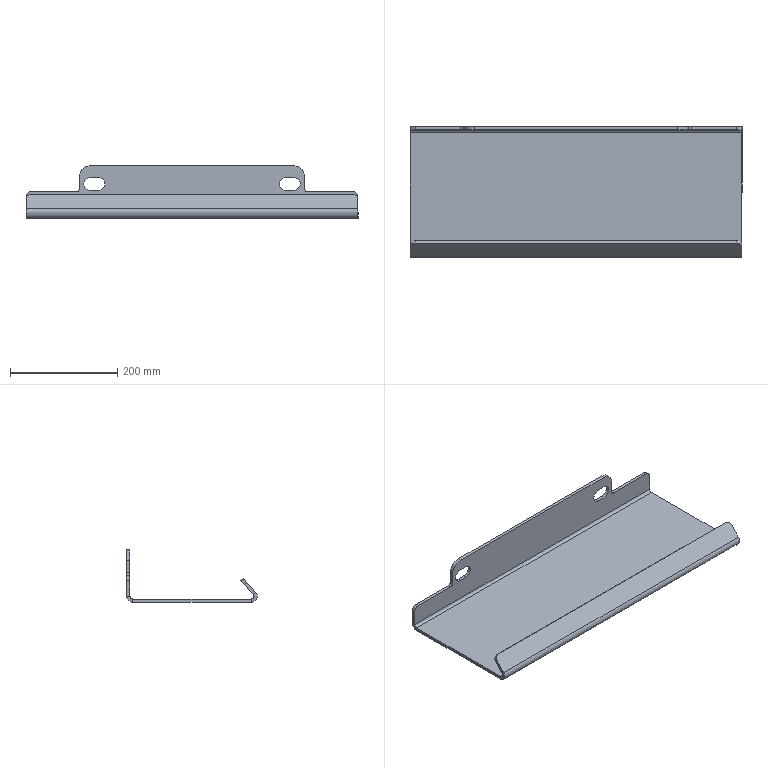Part | SolidWorks | features SM3dBend 2, Fillet 1, FlatPattern 1, SMBaseFlange 1, SheetMetal 1 | 1 solid | 44 faces | box 620 x 243.695 x 98.004 mm | volume 1326121 mm3 | plane 26 | cylinder 18 | commonest cylinder face diameters 24 x6 10 x4 20 x4 22 x2 40 x2
STEP:
#1=CARTESIAN_POINT('',(664.666,380.997,58.004));
#2=VERTEX_POINT('',#1);
#3=CARTESIAN_POINT('',(652.666,380.997,70.004));
#4=VERTEX_POINT('',#3);
#5=CARTESIAN_POINT('',(652.666,380.997,58.004));
#6=DIRECTION('',(0.,-1.,0.));
#7=DIRECTION('',(1.,0.,0.));
#8=AXIS2_PLACEMENT_3D('',#5,#6,#7);
#9=CIRCLE('',#8,12.);
#10=EDGE_CURVE('',#2,#4,#9,.T.);
#11=ORIENTED_EDGE('',*,*,#10,.F.);
#12=CARTESIAN_POINT('',(664.666,374.997,58.004));
#13=VERTEX_POINT('',#12);
#14=CARTESIAN_POINT('',(664.666,380.997,58.004));
#15=DIRECTION('',(0.,-1.,0.));
#16=VECTOR('',#15,1000.);
#17=LINE('',#14,#16);
#18=EDGE_CURVE('',#2,#13,#17,.T.);
#19=ORIENTED_EDGE('',*,*,#18,.T.);
#20=CARTESIAN_POINT('',(652.666,374.997,70.004));
#21=VERTEX_POINT('',#20);
#22=CARTESIAN_POINT('',(652.666,374.997,58.004));
#23=DIRECTION('',(0.,-1.,0.));
#24=DIRECTION('',(1.,0.,0.));
#25=AXIS2_PLACEMENT_3D('',#22,#23,#24);
#26=CIRCLE('',#25,12.);
#27=EDGE_CURVE('',#13,#21,#26,.T.);
#28=ORIENTED_EDGE('',*,*,#27,.T.);
#29=CARTESIAN_POINT('',(652.666,380.997,70.004));
#30=DIRECTION('',(0.,-1.,0.));
#31=VECTOR('',#30,1000.);
#32=LINE('',#29,#31);
#33=EDGE_CURVE('',#4,#21,#32,.T.);
#34=ORIENTED_EDGE('',*,*,#33,.F.);
#35=EDGE_LOOP('',(#11,#19,#28,#34));
#36=FACE_OUTER_BOUND('',#35,.T.);
#37=CARTESIAN_POINT('',(652.666,380.997,58.004));
#38=DIRECTION('',(0.,-1.,0.));
#39=DIRECTION('',(1.,0.,0.));
#40=AXIS2_PLACEMENT_3D('',#37,#38,#39);
#41=CYLINDRICAL_SURFACE('',#40,12.);
#42=ADVANCED_FACE('',(#36),#41,.F.);
#43=CARTESIAN_POINT('',(299.666,380.997,58.004));
#44=VERTEX_POINT('',#43);
#45=CARTESIAN_POINT('',(287.666,380.997,70.004));
#46=VERTEX_POINT('',#45);
#47=CARTESIAN_POINT('',(287.666,380.997,58.004));
#48=DIRECTION('',(0.,-1.,0.));
#49=DIRECTION('',(1.,0.,0.));
#50=AXIS2_PLACEMENT_3D('',#47,#48,#49);
#51=CIRCLE('',#50,12.);
#52=EDGE_CURVE('',#44,#46,#51,.T.);
#53=ORIENTED_EDGE('',*,*,#52,.F.);
#54=CARTESIAN_POINT('',(299.666,374.997,58.004));
#55=VERTEX_POINT('',#54);
#56=CARTESIAN_POINT('',(299.666,380.997,58.004));
#57=DIRECTION('',(0.,-1.,0.));
#58=VECTOR('',#57,1000.);
#59=LINE('',#56,#58);
#60=EDGE_CURVE('',#44,#55,#59,.T.);
#61=ORIENTED_EDGE('',*,*,#60,.T.);
#62=CARTESIAN_POINT('',(287.666,374.997,70.004));
#63=VERTEX_POINT('',#62);
#64=CARTESIAN_POINT('',(287.666,374.997,58.004));
#65=DIRECTION('',(0.,-1.,0.));
#66=DIRECTION('',(1.,0.,0.));
#67=AXIS2_PLACEMENT_3D('',#64,#65,#66);
#68=CIRCLE('',#67,12.);
#69=EDGE_CURVE('',#55,#63,#68,.T.);
#70=ORIENTED_EDGE('',*,*,#69,.T.);
#71=CARTESIAN_POINT('',(287.666,380.997,70.004));
#72=DIRECTION('',(0.,-1.,0.));
#73=VECTOR('',#72,1000.);
#74=LINE('',#71,#73);
#75=EDGE_CURVE('',#46,#63,#74,.T.);
#76=ORIENTED_EDGE('',*,*,#75,.F.);
#77=EDGE_LOOP('',(#53,#61,#70,#76));
#78=FACE_OUTER_BOUND('',#77,.T.);
#79=CARTESIAN_POINT('',(287.666,380.997,58.004));
#80=DIRECTION('',(0.,-1.,0.));
#81=DIRECTION('',(1.,0.,0.));
#82=AXIS2_PLACEMENT_3D('',#79,#80,#81);
#83=CYLINDRICAL_SURFACE('',#82,12.);
#84=ADVANCED_FACE('',(#78),#83,.F.);
#85=CARTESIAN_POINT('',(152.666,369.997,0.));
#86=VERTEX_POINT('',#85);
#87=CARTESIAN_POINT('',(152.666,148.303,0.));
#88=VERTEX_POINT('',#87);
#89=CARTESIAN_POINT('',(152.666,96.654,0.));
#90=DIRECTION('',(0.,-1.,0.));
#91=VECTOR('',#90,1000.);
#92=LINE('',#89,#91);
#93=EDGE_CURVE('',#86,#88,#92,.T.);
#94=ORIENTED_EDGE('',*,*,#93,.F.);
#95=CARTESIAN_POINT('',(152.666,369.997,-6.));
#96=VERTEX_POINT('',#95);
#97=CARTESIAN_POINT('',(152.666,369.997,-6.));
#98=DIRECTION('',(0.,0.,-1.));
#99=VECTOR('',#98,1000.);
#100=LINE('',#97,#99);
#101=EDGE_CURVE('',#86,#96,#100,.T.);
#102=ORIENTED_EDGE('',*,*,#101,.T.);
#103=CARTESIAN_POINT('',(152.666,148.303,-6.));
#104=VERTEX_POINT('',#103);
#105=CARTESIAN_POINT('',(152.666,96.654,-6.));
#106=DIRECTION('',(0.,-1.,0.));
#107=VECTOR('',#106,1000.);
#108=LINE('',#105,#107);
#109=EDGE_CURVE('',#96,#104,#108,.T.);
#110=ORIENTED_EDGE('',*,*,#109,.T.);
#111=CARTESIAN_POINT('',(152.666,148.303,-6.));
#112=DIRECTION('',(0.,0.,-1.));
#113=VECTOR('',#112,1000.);
#114=LINE('',#111,#113);
#115=EDGE_CURVE('',#88,#104,#114,.T.);
#116=ORIENTED_EDGE('',*,*,#115,.F.);
#117=EDGE_LOOP('',(#94,#102,#110,#116));
#118=FACE_OUTER_BOUND('',#117,.T.);
#119=CARTESIAN_POINT('',(152.666,96.654,-6.));
#120=DIRECTION('',(-1.,0.,0.));
#121=DIRECTION('',(0.,0.,1.));
#122=AXIS2_PLACEMENT_3D('',#119,#120,#121);
#123=PLANE('',#122);
#124=ADVANCED_FACE('',(#118),#123,.T.);
#125=CARTESIAN_POINT('',(772.666,148.303,0.));
#126=VERTEX_POINT('',#125);
#127=CARTESIAN_POINT('',(772.666,369.997,0.));
#128=VERTEX_POINT('',#127);
#129=CARTESIAN_POINT('',(772.666,96.654,0.));
#130=DIRECTION('',(0.,1.,0.));
#131=VECTOR('',#130,1000.);
#132=LINE('',#129,#131);
#133=EDGE_CURVE('',#126,#128,#132,.T.);
#134=ORIENTED_EDGE('',*,*,#133,.T.);
#135=CARTESIAN_POINT('',(162.666,369.997,0.));
#136=DIRECTION('',(-1.,0.,0.));
#137=VECTOR('',#136,1000.);
#138=LINE('',#135,#137);
#139=EDGE_CURVE('',#128,#86,#138,.T.);
#140=ORIENTED_EDGE('',*,*,#139,.T.);
#141=ORIENTED_EDGE('',*,*,#93,.T.);
#142=CARTESIAN_POINT('',(162.666,148.303,0.));
#143=DIRECTION('',(-1.,0.,0.));
#144=VECTOR('',#143,1000.);
#145=LINE('',#142,#144);
#146=EDGE_CURVE('',#126,#88,#145,.T.);
#147=ORIENTED_EDGE('',*,*,#146,.F.);
#148=EDGE_LOOP('',(#134,#140,#141,#147));
#149=FACE_OUTER_BOUND('',#148,.T.);
#150=CARTESIAN_POINT('',(162.666,410.154,0.));
#151=DIRECTION('',(0.,0.,1.));
#152=DIRECTION('',(1.,0.,0.));
#153=AXIS2_PLACEMENT_3D('',#150,#151,#152);
#154=PLANE('',#153);
#155=ADVANCED_FACE('',(#149),#154,.T.);
#156=CARTESIAN_POINT('',(772.666,148.303,-6.));
#157=VERTEX_POINT('',#156);
#158=CARTESIAN_POINT('',(772.666,369.997,-6.));
#159=VERTEX_POINT('',#158);
#160=CARTESIAN_POINT('',(772.666,96.654,-6.));
#161=DIRECTION('',(0.,1.,0.));
#162=VECTOR('',#161,1000.);
#163=LINE('',#160,#162);
#164=EDGE_CURVE('',#157,#159,#163,.T.);
#165=ORIENTED_EDGE('',*,*,#164,.T.);
#166=CARTESIAN_POINT('',(772.666,369.997,-6.));
#167=DIRECTION('',(0.,0.,1.));
#168=VECTOR('',#167,1000.);
#169=LINE('',#166,#168);
#170=EDGE_CURVE('',#159,#128,#169,.T.);
#171=ORIENTED_EDGE('',*,*,#170,.T.);
#172=ORIENTED_EDGE('',*,*,#133,.F.);
#173=CARTESIAN_POINT('',(772.666,148.303,-6.));
#174=DIRECTION('',(0.,0.,1.));
#175=VECTOR('',#174,1000.);
#176=LINE('',#173,#175);
#177=EDGE_CURVE('',#157,#126,#176,.T.);
#178=ORIENTED_EDGE('',*,*,#177,.F.);
#179=EDGE_LOOP('',(#165,#171,#172,#178));
#180=FACE_OUTER_BOUND('',#179,.T.);
#181=CARTESIAN_POINT('',(772.666,96.654,-6.));
#182=DIRECTION('',(1.,0.,0.));
#183=DIRECTION('',(0.,0.,-1.));
#184=AXIS2_PLACEMENT_3D('',#181,#182,#183);
#185=PLANE('',#184);
#186=ADVANCED_FACE('',(#180),#185,.T.);
#187=CARTESIAN_POINT('',(772.666,161.51,27.141));
#188=VERTEX_POINT('',#187);
#189=CARTESIAN_POINT('',(772.666,144.587,8.346));
#190=VERTEX_POINT('',#189);
#191=CARTESIAN_POINT('',(772.666,168.202,34.572));
#192=DIRECTION('',(0.,-0.6691,-0.7431));
#193=VECTOR('',#192,1000.);
#194=LINE('',#191,#193);
#195=EDGE_CURVE('',#188,#190,#194,.T.);
#196=ORIENTED_EDGE('',*,*,#195,.F.);
#197=CARTESIAN_POINT('',(772.666,157.051,31.156));
#198=VERTEX_POINT('',#197);
#199=CARTESIAN_POINT('',(772.666,157.051,31.156));
#200=DIRECTION('',(0.,-0.7431,0.6691));
#201=VECTOR('',#200,1000.);
#202=LINE('',#199,#201);
#203=EDGE_CURVE('',#188,#198,#202,.T.);
#204=ORIENTED_EDGE('',*,*,#203,.T.);
#205=CARTESIAN_POINT('',(772.666,140.128,12.36));
#206=VERTEX_POINT('',#205);
#207=CARTESIAN_POINT('',(772.666,163.743,38.587));
#208=DIRECTION('',(0.,-0.6691,-0.7431));
#209=VECTOR('',#208,1000.);
#210=LINE('',#207,#209);
#211=EDGE_CURVE('',#198,#206,#210,.T.);
#212=ORIENTED_EDGE('',*,*,#211,.T.);
#213=CARTESIAN_POINT('',(772.666,140.128,12.36));
#214=DIRECTION('',(0.,0.7431,-0.6691));
#215=VECTOR('',#214,1000.);
#216=LINE('',#213,#215);
#217=EDGE_CURVE('',#206,#190,#216,.T.);
#218=ORIENTED_EDGE('',*,*,#217,.T.);
#219=EDGE_LOOP('',(#196,#204,#212,#218));
#220=FACE_OUTER_BOUND('',#219,.T.);
#221=CARTESIAN_POINT('',(772.666,163.743,38.587));
#222=DIRECTION('',(1.,0.,0.));
#223=DIRECTION('',(0.,-0.7431,0.6691));
#224=AXIS2_PLACEMENT_3D('',#221,#222,#223);
#225=PLANE('',#224);
#226=ADVANCED_FACE('',(#220),#225,.T.);
#227=CARTESIAN_POINT('',(152.666,140.128,12.36));
#228=VERTEX_POINT('',#227);
#229=CARTESIAN_POINT('',(152.666,157.051,31.156));
#230=VERTEX_POINT('',#229);
#231=CARTESIAN_POINT('',(152.666,163.743,38.587));
#232=DIRECTION('',(0.,0.6691,0.7431));
#233=VECTOR('',#232,1000.);
#234=LINE('',#231,#233);
#235=EDGE_CURVE('',#228,#230,#234,.T.);
#236=ORIENTED_EDGE('',*,*,#235,.T.);
#237=CARTESIAN_POINT('',(152.666,161.51,27.141));
#238=VERTEX_POINT('',#237);
#239=CARTESIAN_POINT('',(152.666,157.051,31.156));
#240=DIRECTION('',(0.,0.7431,-0.6691));
#241=VECTOR('',#240,1000.);
#242=LINE('',#239,#241);
#243=EDGE_CURVE('',#230,#238,#242,.T.);
#244=ORIENTED_EDGE('',*,*,#243,.T.);
#245=CARTESIAN_POINT('',(152.666,144.587,8.346));
#246=VERTEX_POINT('',#245);
#247=CARTESIAN_POINT('',(152.666,168.202,34.572));
#248=DIRECTION('',(0.,0.6691,0.7431));
#249=VECTOR('',#248,1000.);
#250=LINE('',#247,#249);
#251=EDGE_CURVE('',#246,#238,#250,.T.);
#252=ORIENTED_EDGE('',*,*,#251,.F.);
#253=CARTESIAN_POINT('',(152.666,140.128,12.36));
#254=DIRECTION('',(0.,-0.7431,0.6691));
#255=VECTOR('',#254,1000.);
#256=LINE('',#253,#255);
#257=EDGE_CURVE('',#246,#228,#256,.T.);
#258=ORIENTED_EDGE('',*,*,#257,.T.);
#259=EDGE_LOOP('',(#236,#244,#252,#258));
#260=FACE_OUTER_BOUND('',#259,.T.);
#261=CARTESIAN_POINT('',(152.666,163.743,38.587));
#262=DIRECTION('',(-1.,0.,0.));
#263=DIRECTION('',(0.,0.7431,-0.6691));
#264=AXIS2_PLACEMENT_3D('',#261,#262,#263);
#265=PLANE('',#264);
#266=ADVANCED_FACE('',(#260),#265,.T.);
#267=CARTESIAN_POINT('',(162.666,168.202,34.572));
#268=VERTEX_POINT('',#267);
#269=CARTESIAN_POINT('',(762.666,168.202,34.572));
#270=VERTEX_POINT('',#269);
#271=CARTESIAN_POINT('',(152.666,168.202,34.572));
#272=DIRECTION('',(1.,0.,0.));
#273=VECTOR('',#272,1000.);
#274=LINE('',#271,#273);
#275=EDGE_CURVE('',#268,#270,#274,.T.);
#276=ORIENTED_EDGE('',*,*,#275,.T.);
#277=CARTESIAN_POINT('',(762.666,161.51,27.141));
#278=DIRECTION('',(0.,0.7431,-0.6691));
#279=DIRECTION('',(0.,0.6691,0.7431));
#280=AXIS2_PLACEMENT_3D('',#277,#278,#279);
#281=CIRCLE('',#280,10.);
#282=EDGE_CURVE('',#270,#188,#281,.T.);
#283=ORIENTED_EDGE('',*,*,#282,.T.);
#284=ORIENTED_EDGE('',*,*,#195,.T.);
#285=CARTESIAN_POINT('',(162.666,144.587,8.346));
#286=DIRECTION('',(-1.,0.,0.));
#287=VECTOR('',#286,1000.);
#288=LINE('',#285,#287);
#289=EDGE_CURVE('',#190,#246,#288,.T.);
#290=ORIENTED_EDGE('',*,*,#289,.T.);
#291=ORIENTED_EDGE('',*,*,#251,.T.);
#292=CARTESIAN_POINT('',(162.666,161.51,27.141));
#293=DIRECTION('',(0.,0.7431,-0.6691));
#294=DIRECTION('',(0.,0.6691,0.7431));
#295=AXIS2_PLACEMENT_3D('',#292,#293,#294);
#296=CIRCLE('',#295,10.);
#297=EDGE_CURVE('',#238,#268,#296,.T.);
#298=ORIENTED_EDGE('',*,*,#297,.T.);
#299=EDGE_LOOP('',(#276,#283,#284,#290,#291,#298));
#300=FACE_OUTER_BOUND('',#299,.T.);
#301=CARTESIAN_POINT('',(162.666,-41.571,-198.403));
#302=DIRECTION('',(0.,0.7431,-0.6691));
#303=DIRECTION('',(1.,0.,0.));
#304=AXIS2_PLACEMENT_3D('',#301,#302,#303);
#305=PLANE('',#304);
#306=ADVANCED_FACE('',(#300),#305,.T.);
#307=CARTESIAN_POINT('',(162.666,163.743,38.587));
#308=VERTEX_POINT('',#307);
#309=CARTESIAN_POINT('',(762.666,163.743,38.587));
#310=VERTEX_POINT('',#309);
#311=CARTESIAN_POINT('',(152.666,163.743,38.587));
#312=DIRECTION('',(1.,0.,0.));
#313=VECTOR('',#312,1000.);
#314=LINE('',#311,#313);
#315=EDGE_CURVE('',#308,#310,#314,.T.);
#316=ORIENTED_EDGE('',*,*,#315,.T.);
#317=CARTESIAN_POINT('',(762.666,163.743,38.587));
#318=DIRECTION('',(0.,0.7431,-0.6691));
#319=VECTOR('',#318,1000.);
#320=LINE('',#317,#319);
#321=EDGE_CURVE('',#310,#270,#320,.T.);
#322=ORIENTED_EDGE('',*,*,#321,.T.);
#323=ORIENTED_EDGE('',*,*,#275,.F.);
#324=CARTESIAN_POINT('',(162.666,163.743,38.587));
#325=DIRECTION('',(0.,-0.7431,0.6691));
#326=VECTOR('',#325,1000.);
#327=LINE('',#324,#326);
#328=EDGE_CURVE('',#268,#308,#327,.T.);
#329=ORIENTED_EDGE('',*,*,#328,.T.);
#330=EDGE_LOOP('',(#316,#322,#323,#329));
#331=FACE_OUTER_BOUND('',#330,.T.);
#332=CARTESIAN_POINT('',(152.666,163.743,38.587));
#333=DIRECTION('',(0.,0.6691,0.7431));
#334=DIRECTION('',(0.,-0.7431,0.6691));
#335=AXIS2_PLACEMENT_3D('',#332,#333,#334);
#336=PLANE('',#335);
#337=ADVANCED_FACE('',(#331),#336,.T.);
#338=ORIENTED_EDGE('',*,*,#211,.F.);
#339=CARTESIAN_POINT('',(762.666,157.051,31.156));
#340=DIRECTION('',(0.,-0.7431,0.6691));
#341=DIRECTION('',(0.,0.6691,0.7431));
#342=AXIS2_PLACEMENT_3D('',#339,#340,#341);
#343=CIRCLE('',#342,10.);
#344=EDGE_CURVE('',#198,#310,#343,.T.);
#345=ORIENTED_EDGE('',*,*,#344,.T.);
#346=ORIENTED_EDGE('',*,*,#315,.F.);
#347=CARTESIAN_POINT('',(162.666,157.051,31.156));
#348=DIRECTION('',(0.,-0.7431,0.6691));
#349=DIRECTION('',(0.,0.6691,0.7431));
#350=AXIS2_PLACEMENT_3D('',#347,#348,#349);
#351=CIRCLE('',#350,10.);
#352=EDGE_CURVE('',#308,#230,#351,.T.);
#353=ORIENTED_EDGE('',*,*,#352,.T.);
#354=ORIENTED_EDGE('',*,*,#235,.F.);
#355=CARTESIAN_POINT('',(162.666,140.128,12.36));
#356=DIRECTION('',(-1.,0.,0.));
#357=VECTOR('',#356,1000.);
#358=LINE('',#355,#357);
#359=EDGE_CURVE('',#206,#228,#358,.T.);
#360=ORIENTED_EDGE('',*,*,#359,.F.);
#361=EDGE_LOOP('',(#338,#345,#346,#353,#354,#360));
#362=FACE_OUTER_BOUND('',#361,.T.);
#363=CARTESIAN_POINT('',(162.666,-46.029,-194.388));
#364=DIRECTION('',(0.,0.7431,-0.6691));
#365=DIRECTION('',(1.,0.,0.));
#366=AXIS2_PLACEMENT_3D('',#363,#364,#365);
#367=PLANE('',#366);
#368=ADVANCED_FACE('',(#362),#367,.F.);
#369=CARTESIAN_POINT('',(162.666,369.997,-6.));
#370=DIRECTION('',(-1.,0.,0.));
#371=VECTOR('',#370,1000.);
#372=LINE('',#369,#371);
#373=EDGE_CURVE('',#159,#96,#372,.T.);
#374=ORIENTED_EDGE('',*,*,#373,.F.);
#375=ORIENTED_EDGE('',*,*,#164,.F.);
#376=CARTESIAN_POINT('',(162.666,148.303,-6.));
#377=DIRECTION('',(-1.,0.,0.));
#378=VECTOR('',#377,1000.);
#379=LINE('',#376,#378);
#380=EDGE_CURVE('',#157,#104,#379,.T.);
#381=ORIENTED_EDGE('',*,*,#380,.T.);
#382=ORIENTED_EDGE('',*,*,#109,.F.);
#383=EDGE_LOOP('',(#374,#375,#381,#382));
#384=FACE_OUTER_BOUND('',#383,.T.);
#385=CARTESIAN_POINT('',(162.666,410.154,-6.));
#386=DIRECTION('',(0.,0.,1.));
#387=DIRECTION('',(1.,0.,0.));
#388=AXIS2_PLACEMENT_3D('',#385,#386,#387);
#389=PLANE('',#388);
#390=ADVANCED_FACE('',(#384),#389,.F.);
#391=ORIENTED_EDGE('',*,*,#177,.T.);
#392=CARTESIAN_POINT('',(772.666,148.303,5.));
#393=DIRECTION('',(-1.,0.,0.));
#394=DIRECTION('',(0.,0.,1.));
#395=AXIS2_PLACEMENT_3D('',#392,#393,#394);
#396=CIRCLE('',#395,5.);
#397=EDGE_CURVE('',#126,#190,#396,.T.);
#398=ORIENTED_EDGE('',*,*,#397,.T.);
#399=ORIENTED_EDGE('',*,*,#217,.F.);
#400=CARTESIAN_POINT('',(772.666,148.303,5.));
#401=DIRECTION('',(-1.,0.,0.));
#402=DIRECTION('',(0.,0.,-1.));
#403=AXIS2_PLACEMENT_3D('',#400,#401,#402);
#404=CIRCLE('',#403,11.);
#405=EDGE_CURVE('',#157,#206,#404,.T.);
#406=ORIENTED_EDGE('',*,*,#405,.F.);
#407=EDGE_LOOP('',(#391,#398,#399,#406));
#408=FACE_OUTER_BOUND('',#407,.T.);
#409=CARTESIAN_POINT('',(772.666,148.303,5.));
#410=DIRECTION('',(1.,0.,0.));
#411=DIRECTION('',(0.,0.,-1.));
#412=AXIS2_PLACEMENT_3D('',#409,#410,#411);
#413=PLANE('',#412);
#414=ADVANCED_FACE('',(#408),#413,.T.);
#415=ORIENTED_EDGE('',*,*,#257,.F.);
#416=CARTESIAN_POINT('',(152.666,148.303,5.));
#417=DIRECTION('',(1.,0.,0.));
#418=DIRECTION('',(0.,0.,1.));
#419=AXIS2_PLACEMENT_3D('',#416,#417,#418);
#420=CIRCLE('',#419,5.);
#421=EDGE_CURVE('',#246,#88,#420,.T.);
#422=ORIENTED_EDGE('',*,*,#421,.T.);
#423=ORIENTED_EDGE('',*,*,#115,.T.);
#424=CARTESIAN_POINT('',(152.666,148.303,5.));
#425=DIRECTION('',(1.,0.,0.));
#426=DIRECTION('',(0.,0.,1.));
#427=AXIS2_PLACEMENT_3D('',#424,#425,#426);
#428=CIRCLE('',#427,11.);
#429=EDGE_CURVE('',#228,#104,#428,.T.);
#430=ORIENTED_EDGE('',*,*,#429,.F.);
#431=EDGE_LOOP('',(#415,#422,#423,#430));
#432=FACE_OUTER_BOUND('',#431,.T.);
#433=CARTESIAN_POINT('',(152.666,148.303,5.));
#434=DIRECTION('',(-1.,0.,0.));
#435=DIRECTION('',(0.,0.,1.));
#436=AXIS2_PLACEMENT_3D('',#433,#434,#435);
#437=PLANE('',#436);
#438=ADVANCED_FACE('',(#432),#437,.T.);
#439=ORIENTED_EDGE('',*,*,#429,.T.);
#440=ORIENTED_EDGE('',*,*,#380,.F.);
#441=ORIENTED_EDGE('',*,*,#405,.T.);
#442=ORIENTED_EDGE('',*,*,#359,.T.);
#443=EDGE_LOOP('',(#439,#440,#441,#442));
#444=FACE_OUTER_BOUND('',#443,.T.);
#445=CARTESIAN_POINT('',(1082.91,148.303,5.));
#446=DIRECTION('',(-1.,0.,0.));
#447=DIRECTION('',(0.,0.,1.));
#448=AXIS2_PLACEMENT_3D('',#445,#446,#447);
#449=CYLINDRICAL_SURFACE('',#448,11.);
#450=ADVANCED_FACE('',(#444),#449,.T.);
#451=ORIENTED_EDGE('',*,*,#421,.F.);
#452=ORIENTED_EDGE('',*,*,#289,.F.);
#453=ORIENTED_EDGE('',*,*,#397,.F.);
#454=ORIENTED_EDGE('',*,*,#146,.T.);
#455=EDGE_LOOP('',(#451,#452,#453,#454));
#456=FACE_OUTER_BOUND('',#455,.T.);
#457=CARTESIAN_POINT('',(1082.91,148.303,5.));
#458=DIRECTION('',(-1.,0.,0.));
#459=DIRECTION('',(0.,0.,1.));
#460=AXIS2_PLACEMENT_3D('',#457,#458,#459);
#461=CYLINDRICAL_SURFACE('',#460,5.);
#462=ADVANCED_FACE('',(#456),#461,.F.);
#463=CARTESIAN_POINT('',(772.666,380.997,5.));
#464=VERTEX_POINT('',#463);
#465=CARTESIAN_POINT('',(772.666,374.997,5.));
#466=VERTEX_POINT('',#465);
#467=CARTESIAN_POINT('',(772.666,380.997,5.));
#468=DIRECTION('',(0.,-1.,0.));
#469=VECTOR('',#468,1000.);
#470=LINE('',#467,#469);
#471=EDGE_CURVE('',#464,#466,#470,.T.);
#472=ORIENTED_EDGE('',*,*,#471,.T.);
#473=CARTESIAN_POINT('',(772.666,369.997,5.));
#474=DIRECTION('',(-1.,0.,0.));
#475=DIRECTION('',(0.,0.,-1.));
#476=AXIS2_PLACEMENT_3D('',#473,#474,#475);
#477=CIRCLE('',#476,5.);
#478=EDGE_CURVE('',#466,#128,#477,.T.);
#479=ORIENTED_EDGE('',*,*,#478,.T.);
#480=ORIENTED_EDGE('',*,*,#170,.F.);
#481=CARTESIAN_POINT('',(772.666,369.997,5.));
#482=DIRECTION('',(-1.,0.,0.));
#483=DIRECTION('',(0.,0.,-1.));
#484=AXIS2_PLACEMENT_3D('',#481,#482,#483);
#485=CIRCLE('',#484,11.);
#486=EDGE_CURVE('',#464,#159,#485,.T.);
#487=ORIENTED_EDGE('',*,*,#486,.F.);
#488=EDGE_LOOP('',(#472,#479,#480,#487));
#489=FACE_OUTER_BOUND('',#488,.T.);
#490=CARTESIAN_POINT('',(772.666,369.997,5.));
#491=DIRECTION('',(1.,0.,0.));
#492=DIRECTION('',(0.,0.,-1.));
#493=AXIS2_PLACEMENT_3D('',#490,#491,#492);
#494=PLANE('',#493);
#495=ADVANCED_FACE('',(#489),#494,.T.);
#496=ORIENTED_EDGE('',*,*,#101,.F.);
#497=CARTESIAN_POINT('',(152.666,374.997,5.));
#498=VERTEX_POINT('',#497);
#499=CARTESIAN_POINT('',(152.666,369.997,5.));
#500=DIRECTION('',(1.,0.,0.));
#501=DIRECTION('',(0.,0.,-1.));
#502=AXIS2_PLACEMENT_3D('',#499,#500,#501);
#503=CIRCLE('',#502,5.);
#504=EDGE_CURVE('',#86,#498,#503,.T.);
#505=ORIENTED_EDGE('',*,*,#504,.T.);
#506=CARTESIAN_POINT('',(152.666,380.997,5.));
#507=VERTEX_POINT('',#506);
#508=CARTESIAN_POINT('',(152.666,380.997,5.));
#509=DIRECTION('',(0.,1.,0.));
#510=VECTOR('',#509,1000.);
#511=LINE('',#508,#510);
#512=EDGE_CURVE('',#498,#507,#511,.T.);
#513=ORIENTED_EDGE('',*,*,#512,.T.);
#514=CARTESIAN_POINT('',(152.666,369.997,5.));
#515=DIRECTION('',(1.,0.,0.));
#516=DIRECTION('',(0.,0.,1.));
#517=AXIS2_PLACEMENT_3D('',#514,#515,#516);
#518=CIRCLE('',#517,11.);
#519=EDGE_CURVE('',#96,#507,#518,.T.);
#520=ORIENTED_EDGE('',*,*,#519,.F.);
#521=EDGE_LOOP('',(#496,#505,#513,#520));
#522=FACE_OUTER_BOUND('',#521,.T.);
#523=CARTESIAN_POINT('',(152.666,369.997,5.));
#524=DIRECTION('',(-1.,0.,0.));
#525=DIRECTION('',(0.,0.,1.));
#526=AXIS2_PLACEMENT_3D('',#523,#524,#525);
#527=PLANE('',#526);
#528=ADVANCED_FACE('',(#522),#527,.T.);
#529=ORIENTED_EDGE('',*,*,#519,.T.);
#530=CARTESIAN_POINT('',(162.666,380.997,5.));
#531=DIRECTION('',(-1.,0.,0.));
#532=VECTOR('',#531,1000.);
#533=LINE('',#530,#532);
#534=EDGE_CURVE('',#464,#507,#533,.T.);
#535=ORIENTED_EDGE('',*,*,#534,.F.);
#536=ORIENTED_EDGE('',*,*,#486,.T.);
#537=ORIENTED_EDGE('',*,*,#373,.T.);
#538=EDGE_LOOP('',(#529,#535,#536,#537));
#539=FACE_OUTER_BOUND('',#538,.T.);
#540=CARTESIAN_POINT('',(-157.464,369.997,5.));
#541=DIRECTION('',(1.,0.,0.));
#542=DIRECTION('',(0.,0.,-1.));
#543=AXIS2_PLACEMENT_3D('',#540,#541,#542);
#544=CYLINDRICAL_SURFACE('',#543,11.);
#545=ADVANCED_FACE('',(#539),#544,.T.);
#546=ORIENTED_EDGE('',*,*,#504,.F.);
#547=ORIENTED_EDGE('',*,*,#139,.F.);
#548=ORIENTED_EDGE('',*,*,#478,.F.);
#549=CARTESIAN_POINT('',(162.666,374.997,5.));
#550=DIRECTION('',(-1.,0.,0.));
#551=VECTOR('',#550,1000.);
#552=LINE('',#549,#551);
#553=EDGE_CURVE('',#466,#498,#552,.T.);
#554=ORIENTED_EDGE('',*,*,#553,.T.);
#555=EDGE_LOOP('',(#546,#547,#548,#554));
#556=FACE_OUTER_BOUND('',#555,.T.);
#557=CARTESIAN_POINT('',(-157.464,369.997,5.));
#558=DIRECTION('',(1.,0.,0.));
#559=DIRECTION('',(0.,0.,-1.));
#560=AXIS2_PLACEMENT_3D('',#557,#558,#559);
#561=CYLINDRICAL_SURFACE('',#560,5.);
#562=ADVANCED_FACE('',(#556),#561,.F.);
#563=CARTESIAN_POINT('',(772.666,374.997,34.004));
#564=VERTEX_POINT('',#563);
#565=CARTESIAN_POINT('',(762.666,374.997,44.004));
#566=VERTEX_POINT('',#565);
#567=CARTESIAN_POINT('',(762.666,374.997,34.004));
#568=DIRECTION('',(0.,-1.,0.));
#569=DIRECTION('',(1.,0.,0.));
#570=AXIS2_PLACEMENT_3D('',#567,#568,#569);
#571=CIRCLE('',#570,10.);
#572=EDGE_CURVE('',#564,#566,#571,.T.);
#573=ORIENTED_EDGE('',*,*,#572,.F.);
#574=CARTESIAN_POINT('',(772.666,380.997,34.004));
#575=VERTEX_POINT('',#574);
#576=CARTESIAN_POINT('',(772.666,380.997,34.004));
#577=DIRECTION('',(0.,-1.,0.));
#578=VECTOR('',#577,1000.);
#579=LINE('',#576,#578);
#580=EDGE_CURVE('',#575,#564,#579,.T.);
#581=ORIENTED_EDGE('',*,*,#580,.F.);
#582=CARTESIAN_POINT('',(762.666,380.997,44.004));
#583=VERTEX_POINT('',#582);
#584=CARTESIAN_POINT('',(762.666,380.997,34.004));
#585=DIRECTION('',(0.,-1.,0.));
#586=DIRECTION('',(1.,0.,0.));
#587=AXIS2_PLACEMENT_3D('',#584,#585,#586);
#588=CIRCLE('',#587,10.);
#589=EDGE_CURVE('',#575,#583,#588,.T.);
#590=ORIENTED_EDGE('',*,*,#589,.T.);
#591=CARTESIAN_POINT('',(762.666,380.997,44.004));
#592=DIRECTION('',(0.,-1.,0.));
#593=VECTOR('',#592,1000.);
#594=LINE('',#591,#593);
#595=EDGE_CURVE('',#583,#566,#594,.T.);
#596=ORIENTED_EDGE('',*,*,#595,.T.);
#597=EDGE_LOOP('',(#573,#581,#590,#596));
#598=FACE_OUTER_BOUND('',#597,.T.);
#599=CARTESIAN_POINT('',(762.666,380.997,34.004));
#600=DIRECTION('',(0.,-1.,0.));
#601=DIRECTION('',(1.,0.,0.));
#602=AXIS2_PLACEMENT_3D('',#599,#600,#601);
#603=CYLINDRICAL_SURFACE('',#602,10.);
#604=ADVANCED_FACE('',(#598),#603,.T.);
#605=CARTESIAN_POINT('',(677.666,374.997,44.004));
#606=VERTEX_POINT('',#605);
#607=CARTESIAN_POINT('',(677.666,374.997,44.004));
#608=DIRECTION('',(-1.,0.,0.));
#609=VECTOR('',#608,1000.);
#610=LINE('',#607,#609);
#611=EDGE_CURVE('',#566,#606,#610,.T.);
#612=ORIENTED_EDGE('',*,*,#611,.F.);
#613=ORIENTED_EDGE('',*,*,#595,.F.);
#614=CARTESIAN_POINT('',(677.666,380.997,44.004));
#615=VERTEX_POINT('',#614);
#616=CARTESIAN_POINT('',(677.666,380.997,44.004));
#617=DIRECTION('',(-1.,0.,0.));
#618=VECTOR('',#617,1000.);
#619=LINE('',#616,#618);
#620=EDGE_CURVE('',#583,#615,#619,.T.);
#621=ORIENTED_EDGE('',*,*,#620,.T.);
#622=CARTESIAN_POINT('',(677.666,380.997,44.004));
#623=DIRECTION('',(0.,-1.,0.));
#624=VECTOR('',#623,1000.);
#625=LINE('',#622,#624);
#626=EDGE_CURVE('',#615,#606,#625,.T.);
#627=ORIENTED_EDGE('',*,*,#626,.T.);
#628=EDGE_LOOP('',(#612,#613,#621,#627));
#629=FACE_OUTER_BOUND('',#628,.T.);
#630=CARTESIAN_POINT('',(677.666,380.997,44.004));
#631=DIRECTION('',(0.,0.,1.));
#632=DIRECTION('',(0.,-1.,0.));
#633=AXIS2_PLACEMENT_3D('',#630,#631,#632);
#634=PLANE('',#633);
#635=ADVANCED_FACE('',(#629),#634,.T.);
#636=CARTESIAN_POINT('',(672.666,374.997,49.004));
#637=VERTEX_POINT('',#636);
#638=CARTESIAN_POINT('',(677.666,374.997,49.004));
#639=DIRECTION('',(0.,1.,0.));
#640=DIRECTION('',(1.,0.,0.));
#641=AXIS2_PLACEMENT_3D('',#638,#639,#640);
#642=CIRCLE('',#641,5.);
#643=EDGE_CURVE('',#606,#637,#642,.T.);
#644=ORIENTED_EDGE('',*,*,#643,.F.);
#645=ORIENTED_EDGE('',*,*,#626,.F.);
#646=CARTESIAN_POINT('',(672.666,380.997,49.004));
#647=VERTEX_POINT('',#646);
#648=CARTESIAN_POINT('',(677.666,380.997,49.004));
#649=DIRECTION('',(0.,1.,0.));
#650=DIRECTION('',(1.,0.,0.));
#651=AXIS2_PLACEMENT_3D('',#648,#649,#650);
#652=CIRCLE('',#651,5.);
#653=EDGE_CURVE('',#615,#647,#652,.T.);
#654=ORIENTED_EDGE('',*,*,#653,.T.);
#655=CARTESIAN_POINT('',(672.666,380.997,49.004));
#656=DIRECTION('',(0.,-1.,0.));
#657=VECTOR('',#656,1000.);
#658=LINE('',#655,#657);
#659=EDGE_CURVE('',#647,#637,#658,.T.);
#660=ORIENTED_EDGE('',*,*,#659,.T.);
#661=EDGE_LOOP('',(#644,#645,#654,#660));
#662=FACE_OUTER_BOUND('',#661,.T.);
#663=CARTESIAN_POINT('',(677.666,380.997,49.004));
#664=DIRECTION('',(0.,-1.,0.));
#665=DIRECTION('',(1.,0.,0.));
#666=AXIS2_PLACEMENT_3D('',#663,#664,#665);
#667=CYLINDRICAL_SURFACE('',#666,5.);
#668=ADVANCED_FACE('',(#662),#667,.F.);
#669=CARTESIAN_POINT('',(672.666,374.997,72.004));
#670=VERTEX_POINT('',#669);
#671=CARTESIAN_POINT('',(672.666,374.997,72.004));
#672=DIRECTION('',(0.,0.,1.));
#673=VECTOR('',#672,1000.);
#674=LINE('',#671,#673);
#675=EDGE_CURVE('',#637,#670,#674,.T.);
#676=ORIENTED_EDGE('',*,*,#675,.F.);
#677=ORIENTED_EDGE('',*,*,#659,.F.);
#678=CARTESIAN_POINT('',(672.666,380.997,72.004));
#679=VERTEX_POINT('',#678);
#680=CARTESIAN_POINT('',(672.666,380.997,72.004));
#681=DIRECTION('',(0.,0.,1.));
#682=VECTOR('',#681,1000.);
#683=LINE('',#680,#682);
#684=EDGE_CURVE('',#647,#679,#683,.T.);
#685=ORIENTED_EDGE('',*,*,#684,.T.);
#686=CARTESIAN_POINT('',(672.666,380.997,72.004));
#687=DIRECTION('',(0.,-1.,0.));
#688=VECTOR('',#687,1000.);
#689=LINE('',#686,#688);
#690=EDGE_CURVE('',#679,#670,#689,.T.);
#691=ORIENTED_EDGE('',*,*,#690,.T.);
#692=EDGE_LOOP('',(#676,#677,#685,#691));
#693=FACE_OUTER_BOUND('',#692,.T.);
#694=CARTESIAN_POINT('',(672.666,380.997,72.004));
#695=DIRECTION('',(1.,0.,0.));
#696=DIRECTION('',(0.,1.,0.));
#697=AXIS2_PLACEMENT_3D('',#694,#695,#696);
#698=PLANE('',#697);
#699=ADVANCED_FACE('',(#693),#698,.T.);
#700=CARTESIAN_POINT('',(652.666,374.997,92.004));
#701=VERTEX_POINT('',#700);
#702=CARTESIAN_POINT('',(652.666,374.997,72.004));
#703=DIRECTION('',(0.,-1.,0.));
#704=DIRECTION('',(1.,0.,0.));
#705=AXIS2_PLACEMENT_3D('',#702,#703,#704);
#706=CIRCLE('',#705,20.);
#707=EDGE_CURVE('',#670,#701,#706,.T.);
#708=ORIENTED_EDGE('',*,*,#707,.F.);
#709=ORIENTED_EDGE('',*,*,#690,.F.);
#710=CARTESIAN_POINT('',(652.666,380.997,92.004));
#711=VERTEX_POINT('',#710);
#712=CARTESIAN_POINT('',(652.666,380.997,72.004));
#713=DIRECTION('',(0.,-1.,0.));
#714=DIRECTION('',(1.,0.,0.));
#715=AXIS2_PLACEMENT_3D('',#712,#713,#714);
#716=CIRCLE('',#715,20.);
#717=EDGE_CURVE('',#679,#711,#716,.T.);
#718=ORIENTED_EDGE('',*,*,#717,.T.);
#719=CARTESIAN_POINT('',(652.666,380.997,92.004));
#720=DIRECTION('',(0.,-1.,0.));
#721=VECTOR('',#720,1000.);
#722=LINE('',#719,#721);
#723=EDGE_CURVE('',#711,#701,#722,.T.);
#724=ORIENTED_EDGE('',*,*,#723,.T.);
#725=EDGE_LOOP('',(#708,#709,#718,#724));
#726=FACE_OUTER_BOUND('',#725,.T.);
#727=CARTESIAN_POINT('',(652.666,380.997,72.004));
#728=DIRECTION('',(0.,-1.,0.));
#729=DIRECTION('',(1.,0.,0.));
#730=AXIS2_PLACEMENT_3D('',#727,#728,#729);
#731=CYLINDRICAL_SURFACE('',#730,20.);
#732=ADVANCED_FACE('',(#726),#731,.T.);
#733=CARTESIAN_POINT('',(272.666,374.997,92.004));
#734=VERTEX_POINT('',#733);
#735=CARTESIAN_POINT('',(272.666,374.997,92.004));
#736=DIRECTION('',(-1.,0.,0.));
#737=VECTOR('',#736,1000.);
#738=LINE('',#735,#737);
#739=EDGE_CURVE('',#701,#734,#738,.T.);
#740=ORIENTED_EDGE('',*,*,#739,.F.);
#741=ORIENTED_EDGE('',*,*,#723,.F.);
#742=CARTESIAN_POINT('',(272.666,380.997,92.004));
#743=VERTEX_POINT('',#742);
#744=CARTESIAN_POINT('',(272.666,380.997,92.004));
#745=DIRECTION('',(-1.,0.,0.));
#746=VECTOR('',#745,1000.);
#747=LINE('',#744,#746);
#748=EDGE_CURVE('',#711,#743,#747,.T.);
#749=ORIENTED_EDGE('',*,*,#748,.T.);
#750=CARTESIAN_POINT('',(272.666,380.997,92.004));
#751=DIRECTION('',(0.,-1.,0.));
#752=VECTOR('',#751,1000.);
#753=LINE('',#750,#752);
#754=EDGE_CURVE('',#743,#734,#753,.T.);
#755=ORIENTED_EDGE('',*,*,#754,.T.);
#756=EDGE_LOOP('',(#740,#741,#749,#755));
#757=FACE_OUTER_BOUND('',#756,.T.);
#758=CARTESIAN_POINT('',(272.666,380.997,92.004));
#759=DIRECTION('',(0.,0.,1.));
#760=DIRECTION('',(0.,-1.,0.));
#761=AXIS2_PLACEMENT_3D('',#758,#759,#760);
#762=PLANE('',#761);
#763=ADVANCED_FACE('',(#757),#762,.T.);
#764=CARTESIAN_POINT('',(252.666,374.997,72.004));
#765=VERTEX_POINT('',#764);
#766=CARTESIAN_POINT('',(272.666,374.997,72.004));
#767=DIRECTION('',(0.,-1.,0.));
#768=DIRECTION('',(1.,0.,0.));
#769=AXIS2_PLACEMENT_3D('',#766,#767,#768);
#770=CIRCLE('',#769,20.);
#771=EDGE_CURVE('',#734,#765,#770,.T.);
#772=ORIENTED_EDGE('',*,*,#771,.F.);
#773=ORIENTED_EDGE('',*,*,#754,.F.);
#774=CARTESIAN_POINT('',(252.666,380.997,72.004));
#775=VERTEX_POINT('',#774);
#776=CARTESIAN_POINT('',(272.666,380.997,72.004));
#777=DIRECTION('',(0.,-1.,0.));
#778=DIRECTION('',(1.,0.,0.));
#779=AXIS2_PLACEMENT_3D('',#776,#777,#778);
#780=CIRCLE('',#779,20.);
#781=EDGE_CURVE('',#743,#775,#780,.T.);
#782=ORIENTED_EDGE('',*,*,#781,.T.);
#783=CARTESIAN_POINT('',(252.666,380.997,72.004));
#784=DIRECTION('',(0.,-1.,0.));
#785=VECTOR('',#784,1000.);
#786=LINE('',#783,#785);
#787=EDGE_CURVE('',#775,#765,#786,.T.);
#788=ORIENTED_EDGE('',*,*,#787,.T.);
#789=EDGE_LOOP('',(#772,#773,#782,#788));
#790=FACE_OUTER_BOUND('',#789,.T.);
#791=CARTESIAN_POINT('',(272.666,380.997,72.004));
#792=DIRECTION('',(0.,-1.,0.));
#793=DIRECTION('',(1.,0.,0.));
#794=AXIS2_PLACEMENT_3D('',#791,#792,#793);
#795=CYLINDRICAL_SURFACE('',#794,20.);
#796=ADVANCED_FACE('',(#790),#795,.T.);
#797=CARTESIAN_POINT('',(252.666,374.997,49.004));
#798=VERTEX_POINT('',#797);
#799=CARTESIAN_POINT('',(252.666,374.997,49.004));
#800=DIRECTION('',(0.,0.,-1.));
#801=VECTOR('',#800,1000.);
#802=LINE('',#799,#801);
#803=EDGE_CURVE('',#765,#798,#802,.T.);
#804=ORIENTED_EDGE('',*,*,#803,.F.);
#805=ORIENTED_EDGE('',*,*,#787,.F.);
#806=CARTESIAN_POINT('',(252.666,380.997,49.004));
#807=VERTEX_POINT('',#806);
#808=CARTESIAN_POINT('',(252.666,380.997,49.004));
#809=DIRECTION('',(0.,0.,-1.));
#810=VECTOR('',#809,1000.);
#811=LINE('',#808,#810);
#812=EDGE_CURVE('',#775,#807,#811,.T.);
#813=ORIENTED_EDGE('',*,*,#812,.T.);
#814=CARTESIAN_POINT('',(252.666,380.997,49.004));
#815=DIRECTION('',(0.,-1.,0.));
#816=VECTOR('',#815,1000.);
#817=LINE('',#814,#816);
#818=EDGE_CURVE('',#807,#798,#817,.T.);
#819=ORIENTED_EDGE('',*,*,#818,.T.);
#820=EDGE_LOOP('',(#804,#805,#813,#819));
#821=FACE_OUTER_BOUND('',#820,.T.);
#822=CARTESIAN_POINT('',(252.666,380.997,49.004));
#823=DIRECTION('',(-1.,0.,0.));
#824=DIRECTION('',(0.,-1.,0.));
#825=AXIS2_PLACEMENT_3D('',#822,#823,#824);
#826=PLANE('',#825);
#827=ADVANCED_FACE('',(#821),#826,.T.);
#828=CARTESIAN_POINT('',(247.666,374.997,44.004));
#829=VERTEX_POINT('',#828);
#830=CARTESIAN_POINT('',(247.666,374.997,49.004));
#831=DIRECTION('',(0.,1.,0.));
#832=DIRECTION('',(1.,0.,0.));
#833=AXIS2_PLACEMENT_3D('',#830,#831,#832);
#834=CIRCLE('',#833,5.);
#835=EDGE_CURVE('',#798,#829,#834,.T.);
#836=ORIENTED_EDGE('',*,*,#835,.F.);
#837=ORIENTED_EDGE('',*,*,#818,.F.);
#838=CARTESIAN_POINT('',(247.666,380.997,44.004));
#839=VERTEX_POINT('',#838);
#840=CARTESIAN_POINT('',(247.666,380.997,49.004));
#841=DIRECTION('',(0.,1.,0.));
#842=DIRECTION('',(1.,0.,0.));
#843=AXIS2_PLACEMENT_3D('',#840,#841,#842);
#844=CIRCLE('',#843,5.);
#845=EDGE_CURVE('',#807,#839,#844,.T.);
#846=ORIENTED_EDGE('',*,*,#845,.T.);
#847=CARTESIAN_POINT('',(247.666,380.997,44.004));
#848=DIRECTION('',(0.,-1.,0.));
#849=VECTOR('',#848,1000.);
#850=LINE('',#847,#849);
#851=EDGE_CURVE('',#839,#829,#850,.T.);
#852=ORIENTED_EDGE('',*,*,#851,.T.);
#853=EDGE_LOOP('',(#836,#837,#846,#852));
#854=FACE_OUTER_BOUND('',#853,.T.);
#855=CARTESIAN_POINT('',(247.666,380.997,49.004));
#856=DIRECTION('',(0.,-1.,0.));
#857=DIRECTION('',(1.,0.,0.));
#858=AXIS2_PLACEMENT_3D('',#855,#856,#857);
#859=CYLINDRICAL_SURFACE('',#858,5.);
#860=ADVANCED_FACE('',(#854),#859,.F.);
#861=CARTESIAN_POINT('',(162.666,374.997,44.004));
#862=VERTEX_POINT('',#861);
#863=CARTESIAN_POINT('',(162.666,374.997,44.004));
#864=DIRECTION('',(-1.,0.,0.));
#865=VECTOR('',#864,1000.);
#866=LINE('',#863,#865);
#867=EDGE_CURVE('',#829,#862,#866,.T.);
#868=ORIENTED_EDGE('',*,*,#867,.F.);
#869=ORIENTED_EDGE('',*,*,#851,.F.);
#870=CARTESIAN_POINT('',(162.666,380.997,44.004));
#871=VERTEX_POINT('',#870);
#872=CARTESIAN_POINT('',(162.666,380.997,44.004));
#873=DIRECTION('',(-1.,0.,0.));
#874=VECTOR('',#873,1000.);
#875=LINE('',#872,#874);
#876=EDGE_CURVE('',#839,#871,#875,.T.);
#877=ORIENTED_EDGE('',*,*,#876,.T.);
#878=CARTESIAN_POINT('',(162.666,380.997,44.004));
#879=DIRECTION('',(0.,-1.,0.));
#880=VECTOR('',#879,1000.);
#881=LINE('',#878,#880);
#882=EDGE_CURVE('',#871,#862,#881,.T.);
#883=ORIENTED_EDGE('',*,*,#882,.T.);
#884=EDGE_LOOP('',(#868,#869,#877,#883));
#885=FACE_OUTER_BOUND('',#884,.T.);
#886=CARTESIAN_POINT('',(162.666,380.997,44.004));
#887=DIRECTION('',(0.,0.,1.));
#888=DIRECTION('',(-1.,0.,0.));
#889=AXIS2_PLACEMENT_3D('',#886,#887,#888);
#890=PLANE('',#889);
#891=ADVANCED_FACE('',(#885),#890,.T.);
#892=CARTESIAN_POINT('',(152.666,374.997,34.004));
#893=VERTEX_POINT('',#892);
#894=CARTESIAN_POINT('',(162.666,374.997,34.004));
#895=DIRECTION('',(0.,-1.,0.));
#896=DIRECTION('',(1.,0.,0.));
#897=AXIS2_PLACEMENT_3D('',#894,#895,#896);
#898=CIRCLE('',#897,10.);
#899=EDGE_CURVE('',#862,#893,#898,.T.);
#900=ORIENTED_EDGE('',*,*,#899,.F.);
#901=ORIENTED_EDGE('',*,*,#882,.F.);
#902=CARTESIAN_POINT('',(152.666,380.997,34.004));
#903=VERTEX_POINT('',#902);
#904=CARTESIAN_POINT('',(162.666,380.997,34.004));
#905=DIRECTION('',(0.,-1.,0.));
#906=DIRECTION('',(1.,0.,0.));
#907=AXIS2_PLACEMENT_3D('',#904,#905,#906);
#908=CIRCLE('',#907,10.);
#909=EDGE_CURVE('',#871,#903,#908,.T.);
#910=ORIENTED_EDGE('',*,*,#909,.T.);
#911=CARTESIAN_POINT('',(152.666,380.997,34.004));
#912=DIRECTION('',(0.,-1.,0.));
#913=VECTOR('',#912,1000.);
#914=LINE('',#911,#913);
#915=EDGE_CURVE('',#903,#893,#914,.T.);
#916=ORIENTED_EDGE('',*,*,#915,.T.);
#917=EDGE_LOOP('',(#900,#901,#910,#916));
#918=FACE_OUTER_BOUND('',#917,.T.);
#919=CARTESIAN_POINT('',(162.666,380.997,34.004));
#920=DIRECTION('',(0.,-1.,0.));
#921=DIRECTION('',(1.,0.,0.));
#922=AXIS2_PLACEMENT_3D('',#919,#920,#921);
#923=CYLINDRICAL_SURFACE('',#922,10.);
#924=ADVANCED_FACE('',(#918),#923,.T.);
#925=CARTESIAN_POINT('',(272.666,374.997,70.004));
#926=VERTEX_POINT('',#925);
#927=CARTESIAN_POINT('',(272.666,374.997,46.004));
#928=VERTEX_POINT('',#927);
#929=CARTESIAN_POINT('',(272.666,374.997,58.004));
#930=DIRECTION('',(0.,-1.,0.));
#931=DIRECTION('',(1.,0.,0.));
#932=AXIS2_PLACEMENT_3D('',#929,#930,#931);
#933=CIRCLE('',#932,12.);
#934=EDGE_CURVE('',#926,#928,#933,.T.);
#935=ORIENTED_EDGE('',*,*,#934,.T.);
#936=CARTESIAN_POINT('',(272.666,380.997,46.004));
#937=VERTEX_POINT('',#936);
#938=CARTESIAN_POINT('',(272.666,380.997,46.004));
#939=DIRECTION('',(0.,-1.,0.));
#940=VECTOR('',#939,1000.);
#941=LINE('',#938,#940);
#942=EDGE_CURVE('',#937,#928,#941,.T.);
#943=ORIENTED_EDGE('',*,*,#942,.F.);
#944=CARTESIAN_POINT('',(272.666,380.997,70.004));
#945=VERTEX_POINT('',#944);
#946=CARTESIAN_POINT('',(272.666,380.997,58.004));
#947=DIRECTION('',(0.,-1.,0.));
#948=DIRECTION('',(1.,0.,0.));
#949=AXIS2_PLACEMENT_3D('',#946,#947,#948);
#950=CIRCLE('',#949,12.);
#951=EDGE_CURVE('',#945,#937,#950,.T.);
#952=ORIENTED_EDGE('',*,*,#951,.F.);
#953=CARTESIAN_POINT('',(272.666,380.997,70.004));
#954=DIRECTION('',(0.,-1.,0.));
#955=VECTOR('',#954,1000.);
#956=LINE('',#953,#955);
#957=EDGE_CURVE('',#945,#926,#956,.T.);
#958=ORIENTED_EDGE('',*,*,#957,.T.);
#959=EDGE_LOOP('',(#935,#943,#952,#958));
#960=FACE_OUTER_BOUND('',#959,.T.);
#961=CARTESIAN_POINT('',(272.666,380.997,58.004));
#962=DIRECTION('',(0.,-1.,0.));
#963=DIRECTION('',(1.,0.,0.));
#964=AXIS2_PLACEMENT_3D('',#961,#962,#963);
#965=CYLINDRICAL_SURFACE('',#964,12.);
#966=ADVANCED_FACE('',(#960),#965,.F.);
#967=CARTESIAN_POINT('',(287.666,374.997,70.004));
#968=DIRECTION('',(-1.,0.,0.));
#969=VECTOR('',#968,1000.);
#970=LINE('',#967,#969);
#971=EDGE_CURVE('',#63,#926,#970,.T.);
#972=ORIENTED_EDGE('',*,*,#971,.T.);
#973=ORIENTED_EDGE('',*,*,#957,.F.);
#974=CARTESIAN_POINT('',(287.666,380.997,70.004));
#975=DIRECTION('',(-1.,0.,0.));
#976=VECTOR('',#975,1000.);
#977=LINE('',#974,#976);
#978=EDGE_CURVE('',#46,#945,#977,.T.);
#979=ORIENTED_EDGE('',*,*,#978,.F.);
#980=ORIENTED_EDGE('',*,*,#75,.T.);
#981=EDGE_LOOP('',(#972,#973,#979,#980));
#982=FACE_OUTER_BOUND('',#981,.T.);
#983=CARTESIAN_POINT('',(287.666,380.997,70.004));
#984=DIRECTION('',(0.,0.,1.));
#985=DIRECTION('',(0.,-1.,0.));
#986=AXIS2_PLACEMENT_3D('',#983,#984,#985);
#987=PLANE('',#986);
#988=ADVANCED_FACE('',(#982),#987,.F.);
#989=ORIENTED_EDGE('',*,*,#60,.F.);
#990=CARTESIAN_POINT('',(287.666,380.997,46.004));
#991=VERTEX_POINT('',#990);
#992=CARTESIAN_POINT('',(287.666,380.997,58.004));
#993=DIRECTION('',(0.,-1.,0.));
#994=DIRECTION('',(1.,0.,0.));
#995=AXIS2_PLACEMENT_3D('',#992,#993,#994);
#996=CIRCLE('',#995,12.);
#997=EDGE_CURVE('',#991,#44,#996,.T.);
#998=ORIENTED_EDGE('',*,*,#997,.F.);
#999=CARTESIAN_POINT('',(287.666,374.997,46.004));
#1000=VERTEX_POINT('',#999);
#1001=CARTESIAN_POINT('',(287.666,380.997,46.004));
#1002=DIRECTION('',(0.,-1.,0.));
#1003=VECTOR('',#1002,1000.);
#1004=LINE('',#1001,#1003);
#1005=EDGE_CURVE('',#991,#1000,#1004,.T.);
#1006=ORIENTED_EDGE('',*,*,#1005,.T.);
#1007=CARTESIAN_POINT('',(287.666,374.997,58.004));
#1008=DIRECTION('',(0.,-1.,0.));
#1009=DIRECTION('',(1.,0.,0.));
#1010=AXIS2_PLACEMENT_3D('',#1007,#1008,#1009);
#1011=CIRCLE('',#1010,12.);
#1012=EDGE_CURVE('',#1000,#55,#1011,.T.);
#1013=ORIENTED_EDGE('',*,*,#1012,.T.);
#1014=EDGE_LOOP('',(#989,#998,#1006,#1013));
#1015=FACE_OUTER_BOUND('',#1014,.T.);
#1016=CARTESIAN_POINT('',(287.666,380.997,58.004));
#1017=DIRECTION('',(0.,-1.,0.));
#1018=DIRECTION('',(1.,0.,0.));
#1019=AXIS2_PLACEMENT_3D('',#1016,#1017,#1018);
#1020=CYLINDRICAL_SURFACE('',#1019,12.);
#1021=ADVANCED_FACE('',(#1015),#1020,.F.);
#1022=CARTESIAN_POINT('',(272.666,374.997,46.004));
#1023=DIRECTION('',(1.,0.,0.));
#1024=VECTOR('',#1023,1000.);
#1025=LINE('',#1022,#1024);
#1026=EDGE_CURVE('',#928,#1000,#1025,.T.);
#1027=ORIENTED_EDGE('',*,*,#1026,.T.);
#1028=ORIENTED_EDGE('',*,*,#1005,.F.);
#1029=CARTESIAN_POINT('',(272.666,380.997,46.004));
#1030=DIRECTION('',(1.,0.,0.));
#1031=VECTOR('',#1030,1000.);
#1032=LINE('',#1029,#1031);
#1033=EDGE_CURVE('',#937,#991,#1032,.T.);
#1034=ORIENTED_EDGE('',*,*,#1033,.F.);
#1035=ORIENTED_EDGE('',*,*,#942,.T.);
#1036=EDGE_LOOP('',(#1027,#1028,#1034,#1035));
#1037=FACE_OUTER_BOUND('',#1036,.T.);
#1038=CARTESIAN_POINT('',(272.666,380.997,46.004));
#1039=DIRECTION('',(0.,0.,-1.));
#1040=DIRECTION('',(1.,0.,0.));
#1041=AXIS2_PLACEMENT_3D('',#1038,#1039,#1040);
#1042=PLANE('',#1041);
#1043=ADVANCED_FACE('',(#1037),#1042,.F.);
#1044=CARTESIAN_POINT('',(637.666,374.997,70.004));
#1045=VERTEX_POINT('',#1044);
#1046=CARTESIAN_POINT('',(637.666,374.997,46.004));
#1047=VERTEX_POINT('',#1046);
#1048=CARTESIAN_POINT('',(637.666,374.997,58.004));
#1049=DIRECTION('',(0.,-1.,0.));
#1050=DIRECTION('',(1.,0.,0.));
#1051=AXIS2_PLACEMENT_3D('',#1048,#1049,#1050);
#1052=CIRCLE('',#1051,12.);
#1053=EDGE_CURVE('',#1045,#1047,#1052,.T.);
#1054=ORIENTED_EDGE('',*,*,#1053,.T.);
#1055=CARTESIAN_POINT('',(637.666,380.997,46.004));
#1056=VERTEX_POINT('',#1055);
#1057=CARTESIAN_POINT('',(637.666,380.997,46.004));
#1058=DIRECTION('',(0.,-1.,0.));
#1059=VECTOR('',#1058,1000.);
#1060=LINE('',#1057,#1059);
#1061=EDGE_CURVE('',#1056,#1047,#1060,.T.);
#1062=ORIENTED_EDGE('',*,*,#1061,.F.);
#1063=CARTESIAN_POINT('',(637.666,380.997,70.004));
#1064=VERTEX_POINT('',#1063);
#1065=CARTESIAN_POINT('',(637.666,380.997,58.004));
#1066=DIRECTION('',(0.,-1.,0.));
#1067=DIRECTION('',(1.,0.,0.));
#1068=AXIS2_PLACEMENT_3D('',#1065,#1066,#1067);
#1069=CIRCLE('',#1068,12.);
#1070=EDGE_CURVE('',#1064,#1056,#1069,.T.);
#1071=ORIENTED_EDGE('',*,*,#1070,.F.);
#1072=CARTESIAN_POINT('',(637.666,380.997,70.004));
#1073=DIRECTION('',(0.,-1.,0.));
#1074=VECTOR('',#1073,1000.);
#1075=LINE('',#1072,#1074);
#1076=EDGE_CURVE('',#1064,#1045,#1075,.T.);
#1077=ORIENTED_EDGE('',*,*,#1076,.T.);
#1078=EDGE_LOOP('',(#1054,#1062,#1071,#1077));
#1079=FACE_OUTER_BOUND('',#1078,.T.);
#1080=CARTESIAN_POINT('',(637.666,380.997,58.004));
#1081=DIRECTION('',(0.,-1.,0.));
#1082=DIRECTION('',(1.,0.,0.));
#1083=AXIS2_PLACEMENT_3D('',#1080,#1081,#1082);
#1084=CYLINDRICAL_SURFACE('',#1083,12.);
#1085=ADVANCED_FACE('',(#1079),#1084,.F.);
#1086=CARTESIAN_POINT('',(652.666,374.997,70.004));
#1087=DIRECTION('',(-1.,0.,0.));
#1088=VECTOR('',#1087,1000.);
#1089=LINE('',#1086,#1088);
#1090=EDGE_CURVE('',#21,#1045,#1089,.T.);
#1091=ORIENTED_EDGE('',*,*,#1090,.T.);
#1092=ORIENTED_EDGE('',*,*,#1076,.F.);
#1093=CARTESIAN_POINT('',(652.666,380.997,70.004));
#1094=DIRECTION('',(-1.,0.,0.));
#1095=VECTOR('',#1094,1000.);
#1096=LINE('',#1093,#1095);
#1097=EDGE_CURVE('',#4,#1064,#1096,.T.);
#1098=ORIENTED_EDGE('',*,*,#1097,.F.);
#1099=ORIENTED_EDGE('',*,*,#33,.T.);
#1100=EDGE_LOOP('',(#1091,#1092,#1098,#1099));
#1101=FACE_OUTER_BOUND('',#1100,.T.);
#1102=CARTESIAN_POINT('',(652.666,380.997,70.004));
#1103=DIRECTION('',(0.,0.,1.));
#1104=DIRECTION('',(-1.,0.,0.));
#1105=AXIS2_PLACEMENT_3D('',#1102,#1103,#1104);
#1106=PLANE('',#1105);
#1107=ADVANCED_FACE('',(#1101),#1106,.F.);
#1108=ORIENTED_EDGE('',*,*,#18,.F.);
#1109=CARTESIAN_POINT('',(652.666,380.997,46.004));
#1110=VERTEX_POINT('',#1109);
#1111=CARTESIAN_POINT('',(652.666,380.997,58.004));
#1112=DIRECTION('',(0.,-1.,0.));
#1113=DIRECTION('',(1.,0.,0.));
#1114=AXIS2_PLACEMENT_3D('',#1111,#1112,#1113);
#1115=CIRCLE('',#1114,12.);
#1116=EDGE_CURVE('',#1110,#2,#1115,.T.);
#1117=ORIENTED_EDGE('',*,*,#1116,.F.);
#1118=CARTESIAN_POINT('',(652.666,374.997,46.004));
#1119=VERTEX_POINT('',#1118);
#1120=CARTESIAN_POINT('',(652.666,380.997,46.004));
#1121=DIRECTION('',(0.,-1.,0.));
#1122=VECTOR('',#1121,1000.);
#1123=LINE('',#1120,#1122);
#1124=EDGE_CURVE('',#1110,#1119,#1123,.T.);
#1125=ORIENTED_EDGE('',*,*,#1124,.T.);
#1126=CARTESIAN_POINT('',(652.666,374.997,58.004));
#1127=DIRECTION('',(0.,-1.,0.));
#1128=DIRECTION('',(1.,0.,0.));
#1129=AXIS2_PLACEMENT_3D('',#1126,#1127,#1128);
#1130=CIRCLE('',#1129,12.);
#1131=EDGE_CURVE('',#1119,#13,#1130,.T.);
#1132=ORIENTED_EDGE('',*,*,#1131,.T.);
#1133=EDGE_LOOP('',(#1108,#1117,#1125,#1132));
#1134=FACE_OUTER_BOUND('',#1133,.T.);
#1135=CARTESIAN_POINT('',(652.666,380.997,58.004));
#1136=DIRECTION('',(0.,-1.,0.));
#1137=DIRECTION('',(1.,0.,0.));
#1138=AXIS2_PLACEMENT_3D('',#1135,#1136,#1137);
#1139=CYLINDRICAL_SURFACE('',#1138,12.);
#1140=ADVANCED_FACE('',(#1134),#1139,.F.);
#1141=CARTESIAN_POINT('',(637.666,374.997,46.004));
#1142=DIRECTION('',(1.,0.,0.));
#1143=VECTOR('',#1142,1000.);
#1144=LINE('',#1141,#1143);
#1145=EDGE_CURVE('',#1047,#1119,#1144,.T.);
#1146=ORIENTED_EDGE('',*,*,#1145,.T.);
#1147=ORIENTED_EDGE('',*,*,#1124,.F.);
#1148=CARTESIAN_POINT('',(637.666,380.997,46.004));
#1149=DIRECTION('',(1.,0.,0.));
#1150=VECTOR('',#1149,1000.);
#1151=LINE('',#1148,#1150);
#1152=EDGE_CURVE('',#1056,#1110,#1151,.T.);
#1153=ORIENTED_EDGE('',*,*,#1152,.F.);
#1154=ORIENTED_EDGE('',*,*,#1061,.T.);
#1155=EDGE_LOOP('',(#1146,#1147,#1153,#1154));
#1156=FACE_OUTER_BOUND('',#1155,.T.);
#1157=CARTESIAN_POINT('',(637.666,380.997,46.004));
#1158=DIRECTION('',(0.,0.,-1.));
#1159=DIRECTION('',(1.,0.,0.));
#1160=AXIS2_PLACEMENT_3D('',#1157,#1158,#1159);
#1161=PLANE('',#1160);
#1162=ADVANCED_FACE('',(#1156),#1161,.F.);
#1163=ORIENTED_EDGE('',*,*,#1152,.T.);
#1164=ORIENTED_EDGE('',*,*,#1116,.T.);
#1165=ORIENTED_EDGE('',*,*,#10,.T.);
#1166=ORIENTED_EDGE('',*,*,#1097,.T.);
#1167=ORIENTED_EDGE('',*,*,#1070,.T.);
#1168=EDGE_LOOP('',(#1163,#1164,#1165,#1166,#1167));
#1169=FACE_BOUND('',#1168,.T.);
#1170=ORIENTED_EDGE('',*,*,#1033,.T.);
#1171=ORIENTED_EDGE('',*,*,#997,.T.);
#1172=ORIENTED_EDGE('',*,*,#52,.T.);
#1173=ORIENTED_EDGE('',*,*,#978,.T.);
#1174=ORIENTED_EDGE('',*,*,#951,.T.);
#1175=EDGE_LOOP('',(#1170,#1171,#1172,#1173,#1174));
#1176=FACE_BOUND('',#1175,.T.);
#1177=CARTESIAN_POINT('',(772.666,380.997,-279.496));
#1178=DIRECTION('',(0.,0.,1.));
#1179=VECTOR('',#1178,1000.);
#1180=LINE('',#1177,#1179);
#1181=EDGE_CURVE('',#464,#575,#1180,.T.);
#1182=ORIENTED_EDGE('',*,*,#1181,.F.);
#1183=ORIENTED_EDGE('',*,*,#534,.T.);
#1184=CARTESIAN_POINT('',(152.666,380.997,-279.496));
#1185=DIRECTION('',(0.,0.,-1.));
#1186=VECTOR('',#1185,1000.);
#1187=LINE('',#1184,#1186);
#1188=EDGE_CURVE('',#903,#507,#1187,.T.);
#1189=ORIENTED_EDGE('',*,*,#1188,.F.);
#1190=ORIENTED_EDGE('',*,*,#909,.F.);
#1191=ORIENTED_EDGE('',*,*,#876,.F.);
#1192=ORIENTED_EDGE('',*,*,#845,.F.);
#1193=ORIENTED_EDGE('',*,*,#812,.F.);
#1194=ORIENTED_EDGE('',*,*,#781,.F.);
#1195=ORIENTED_EDGE('',*,*,#748,.F.);
#1196=ORIENTED_EDGE('',*,*,#717,.F.);
#1197=ORIENTED_EDGE('',*,*,#684,.F.);
#1198=ORIENTED_EDGE('',*,*,#653,.F.);
#1199=ORIENTED_EDGE('',*,*,#620,.F.);
#1200=ORIENTED_EDGE('',*,*,#589,.F.);
#1201=EDGE_LOOP('',(#1182,#1183,#1189,#1190,#1191,#1192,#1193,#1194,#1195,#1196,#1197,#1198,#1199,#1200));
#1202=FACE_OUTER_BOUND('',#1201,.T.);
#1203=CARTESIAN_POINT('',(162.666,380.997,34.004));
#1204=DIRECTION('',(0.,-1.,0.));
#1205=DIRECTION('',(1.,0.,0.));
#1206=AXIS2_PLACEMENT_3D('',#1203,#1204,#1205);
#1207=PLANE('',#1206);
#1208=ADVANCED_FACE('',(#1169,#1176,#1202),#1207,.F.);
#1209=ORIENTED_EDGE('',*,*,#512,.F.);
#1210=CARTESIAN_POINT('',(152.666,374.997,-279.496));
#1211=DIRECTION('',(0.,0.,-1.));
#1212=VECTOR('',#1211,1000.);
#1213=LINE('',#1210,#1212);
#1214=EDGE_CURVE('',#893,#498,#1213,.T.);
#1215=ORIENTED_EDGE('',*,*,#1214,.F.);
#1216=ORIENTED_EDGE('',*,*,#915,.F.);
#1217=ORIENTED_EDGE('',*,*,#1188,.T.);
#1218=EDGE_LOOP('',(#1209,#1215,#1216,#1217));
#1219=FACE_OUTER_BOUND('',#1218,.T.);
#1220=CARTESIAN_POINT('',(152.666,380.997,-279.496));
#1221=DIRECTION('',(-1.,0.,0.));
#1222=DIRECTION('',(0.,-1.,0.));
#1223=AXIS2_PLACEMENT_3D('',#1220,#1221,#1222);
#1224=PLANE('',#1223);
#1225=ADVANCED_FACE('',(#1219),#1224,.T.);
#1226=ORIENTED_EDGE('',*,*,#553,.F.);
#1227=CARTESIAN_POINT('',(772.666,374.997,-279.496));
#1228=DIRECTION('',(0.,0.,1.));
#1229=VECTOR('',#1228,1000.);
#1230=LINE('',#1227,#1229);
#1231=EDGE_CURVE('',#466,#564,#1230,.T.);
#1232=ORIENTED_EDGE('',*,*,#1231,.T.);
#1233=ORIENTED_EDGE('',*,*,#572,.T.);
#1234=ORIENTED_EDGE('',*,*,#611,.T.);
#1235=ORIENTED_EDGE('',*,*,#643,.T.);
#1236=ORIENTED_EDGE('',*,*,#675,.T.);
#1237=ORIENTED_EDGE('',*,*,#707,.T.);
#1238=ORIENTED_EDGE('',*,*,#739,.T.);
#1239=ORIENTED_EDGE('',*,*,#771,.T.);
#1240=ORIENTED_EDGE('',*,*,#803,.T.);
#1241=ORIENTED_EDGE('',*,*,#835,.T.);
#1242=ORIENTED_EDGE('',*,*,#867,.T.);
#1243=ORIENTED_EDGE('',*,*,#899,.T.);
#1244=ORIENTED_EDGE('',*,*,#1214,.T.);
#1245=EDGE_LOOP('',(#1226,#1232,#1233,#1234,#1235,#1236,#1237,#1238,#1239,#1240,#1241,#1242,#1243,#1244));
#1246=FACE_OUTER_BOUND('',#1245,.T.);
#1247=ORIENTED_EDGE('',*,*,#1131,.F.);
#1248=ORIENTED_EDGE('',*,*,#1145,.F.);
#1249=ORIENTED_EDGE('',*,*,#1053,.F.);
#1250=ORIENTED_EDGE('',*,*,#1090,.F.);
#1251=ORIENTED_EDGE('',*,*,#27,.F.);
#1252=EDGE_LOOP('',(#1247,#1248,#1249,#1250,#1251));
#1253=FACE_BOUND('',#1252,.T.);
#1254=ORIENTED_EDGE('',*,*,#1012,.F.);
#1255=ORIENTED_EDGE('',*,*,#1026,.F.);
#1256=ORIENTED_EDGE('',*,*,#934,.F.);
#1257=ORIENTED_EDGE('',*,*,#971,.F.);
#1258=ORIENTED_EDGE('',*,*,#69,.F.);
#1259=EDGE_LOOP('',(#1254,#1255,#1256,#1257,#1258));
#1260=FACE_BOUND('',#1259,.T.);
#1261=CARTESIAN_POINT('',(162.666,374.997,34.004));
#1262=DIRECTION('',(0.,-1.,0.));
#1263=DIRECTION('',(1.,0.,0.));
#1264=AXIS2_PLACEMENT_3D('',#1261,#1262,#1263);
#1265=PLANE('',#1264);
#1266=ADVANCED_FACE('',(#1246,#1253,#1260),#1265,.T.);
#1267=ORIENTED_EDGE('',*,*,#471,.F.);
#1268=ORIENTED_EDGE('',*,*,#1181,.T.);
#1269=ORIENTED_EDGE('',*,*,#580,.T.);
#1270=ORIENTED_EDGE('',*,*,#1231,.F.);
#1271=EDGE_LOOP('',(#1267,#1268,#1269,#1270));
#1272=FACE_OUTER_BOUND('',#1271,.T.);
#1273=CARTESIAN_POINT('',(772.666,380.997,-279.496));
#1274=DIRECTION('',(1.,0.,0.));
#1275=DIRECTION('',(0.,1.,0.));
#1276=AXIS2_PLACEMENT_3D('',#1273,#1274,#1275);
#1277=PLANE('',#1276);
#1278=ADVANCED_FACE('',(#1272),#1277,.T.);
#1279=ORIENTED_EDGE('',*,*,#344,.F.);
#1280=ORIENTED_EDGE('',*,*,#203,.F.);
#1281=ORIENTED_EDGE('',*,*,#282,.F.);
#1282=ORIENTED_EDGE('',*,*,#321,.F.);
#1283=EDGE_LOOP('',(#1279,#1280,#1281,#1282));
#1284=FACE_OUTER_BOUND('',#1283,.T.);
#1285=CARTESIAN_POINT('',(762.666,157.051,31.156));
#1286=DIRECTION('',(0.,0.7431,-0.6691));
#1287=DIRECTION('',(0.,0.6691,0.7431));
#1288=AXIS2_PLACEMENT_3D('',#1285,#1286,#1287);
#1289=CYLINDRICAL_SURFACE('',#1288,10.);
#1290=ADVANCED_FACE('',(#1284),#1289,.T.);
#1291=ORIENTED_EDGE('',*,*,#352,.F.);
#1292=ORIENTED_EDGE('',*,*,#328,.F.);
#1293=ORIENTED_EDGE('',*,*,#297,.F.);
#1294=ORIENTED_EDGE('',*,*,#243,.F.);
#1295=EDGE_LOOP('',(#1291,#1292,#1293,#1294));
#1296=FACE_OUTER_BOUND('',#1295,.T.);
#1297=CARTESIAN_POINT('',(162.666,157.051,31.156));
#1298=DIRECTION('',(0.,0.7431,-0.6691));
#1299=DIRECTION('',(0.,0.6691,0.7431));
#1300=AXIS2_PLACEMENT_3D('',#1297,#1298,#1299);
#1301=CYLINDRICAL_SURFACE('',#1300,10.);
#1302=ADVANCED_FACE('',(#1296),#1301,.T.);
#1303=CLOSED_SHELL('',(#42,#84,#124,#155,#186,#226,#266,#306,#337,#368,#390,#414,#438,#450,#462,#495,#528,#545,#562,#604,#635,#668,#699,#732,#763,#796,#827,#860,#891,#924,#966,#988,#1021,#1043,#1085,#1107,#1140,#1162,#1208,#1225,#1266,#1278,#1290,#1302));
#1304=MANIFOLD_SOLID_BREP('',#1303);
#1305=CARTESIAN_POINT('',(0.,0.,0.));
#1306=DIRECTION('',(0.,0.,1.));
#1307=DIRECTION('',(1.,0.,0.));
#1308=AXIS2_PLACEMENT_3D('',#1305,#1306,#1307);
#1309=(LENGTH_UNIT()NAMED_UNIT(*)SI_UNIT(.MILLI.,.METRE.));
#1310=UNCERTAINTY_MEASURE_WITH_UNIT(LENGTH_MEASURE(0.00001),#1309,'','');
#1311=(NAMED_UNIT(*)PLANE_ANGLE_UNIT()SI_UNIT($,.RADIAN.));
#1312=(NAMED_UNIT(*)SI_UNIT($,.STERADIAN.)SOLID_ANGLE_UNIT());
#1313=(GEOMETRIC_REPRESENTATION_CONTEXT(3)GLOBAL_UNCERTAINTY_ASSIGNED_CONTEXT((#1310))GLOBAL_UNIT_ASSIGNED_CONTEXT((#1309,#1311,#1312))REPRESENTATION_CONTEXT('',''));
#1314=ADVANCED_BREP_SHAPE_REPRESENTATION('',(#1304,#1308),#1313);